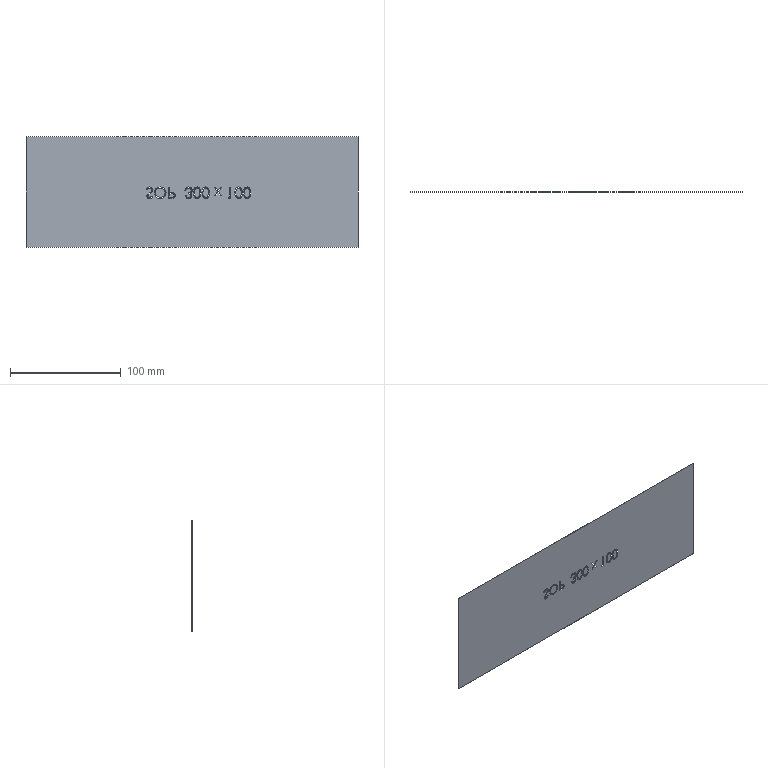Part | NX | features BREP 7 | 7 solids | 128 faces | box 300 x 0.1 x 100 mm | volume 2979 mm3 | spline 79 | plane 49